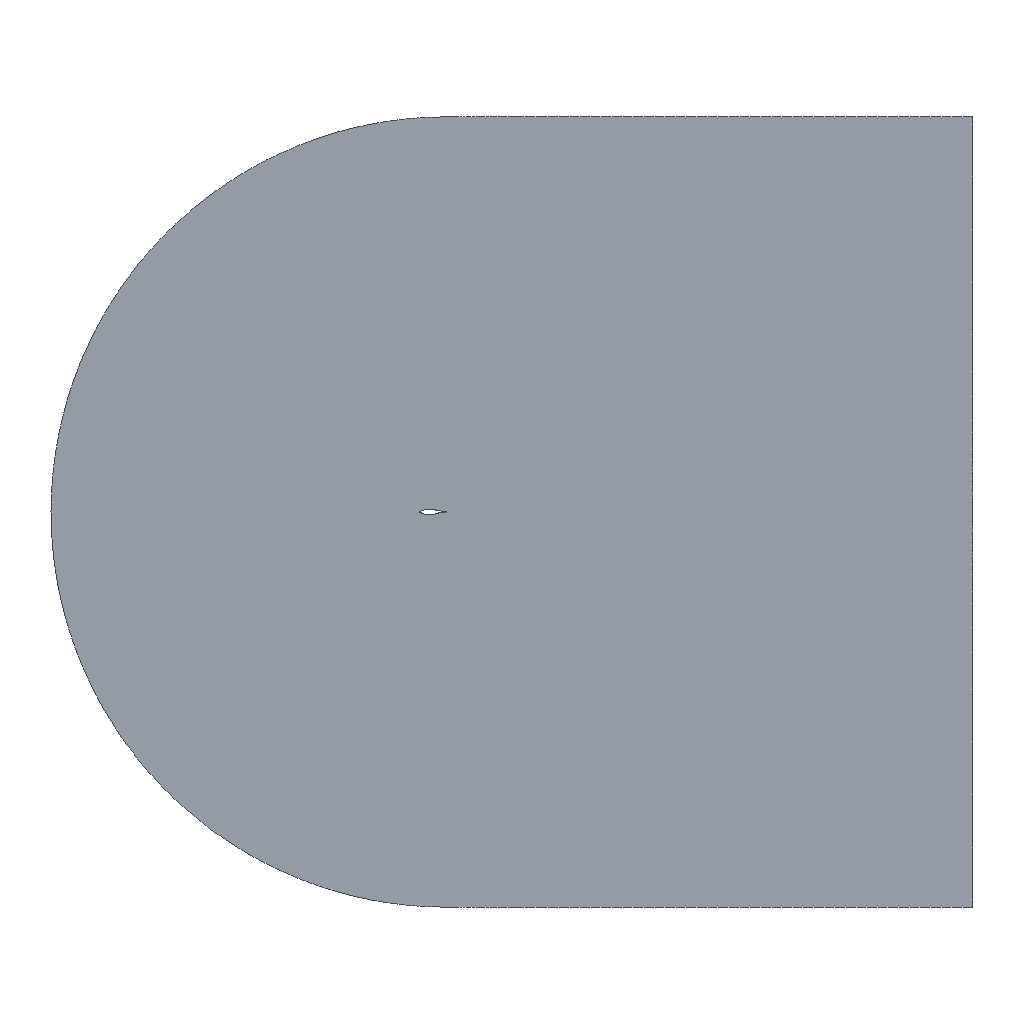Simulation study | ansys fluent
Set-up summary:
category,name,step,type,value,unit,region
solver,ansys_fluent
units,not stated in the deck,,not stated
analysis,deck,,Steady,Steady
physics,Time,,model,Steady
physics,Space,,model,2D
physics,Species,,model,Disabled
physics,Viscous,,model,SST k-omega turbulence model
physics,Structure,,model,Disabled
physics,Multiphase,,model,Disabled
physics,Heat Transfer,,model,Disabled
material,air,,fluid
material,aluminum,,solid
bc,outlet,,pressure-outlet
bc,airfoil_up,,wall
bc,airfoil_down,,wall
bc,velocity_inlet,,velocity-inlet
Results summary:
result,analysis,,,Steady
result,pressure,,min/max,-12.649 / 15.161
result,velocity-magnitude,,min/max,0.001147 / 6.713
result,turb-kinetic-energy,,min/max,2.942732e-08 / 0.4991